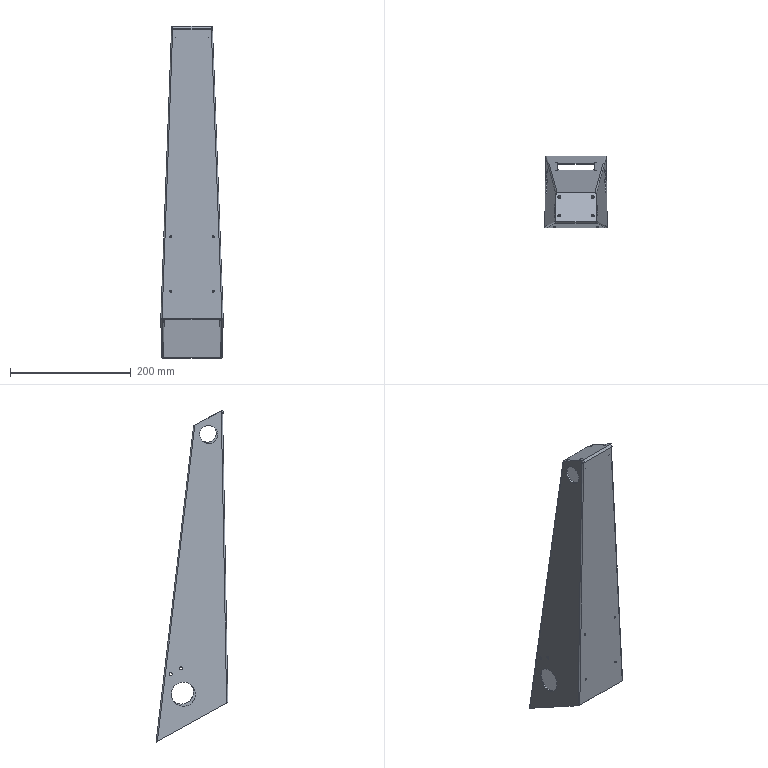Part | SolidWorks | features HoleWzd 4, Fillet 3, Cut 2, ICE 2, Blend 1, MirrorPattern 1, Shell 1 | 1 solid | 81 faces | box 103.468 x 118.808 x 550 mm | volume 320193 mm3 | cylinder 53 | plane 20 | cone 4 | spline 4 | commonest cylinder face diameters 5 x20 3.3 x16 4 x5 10 x4 30 x4 40 x4